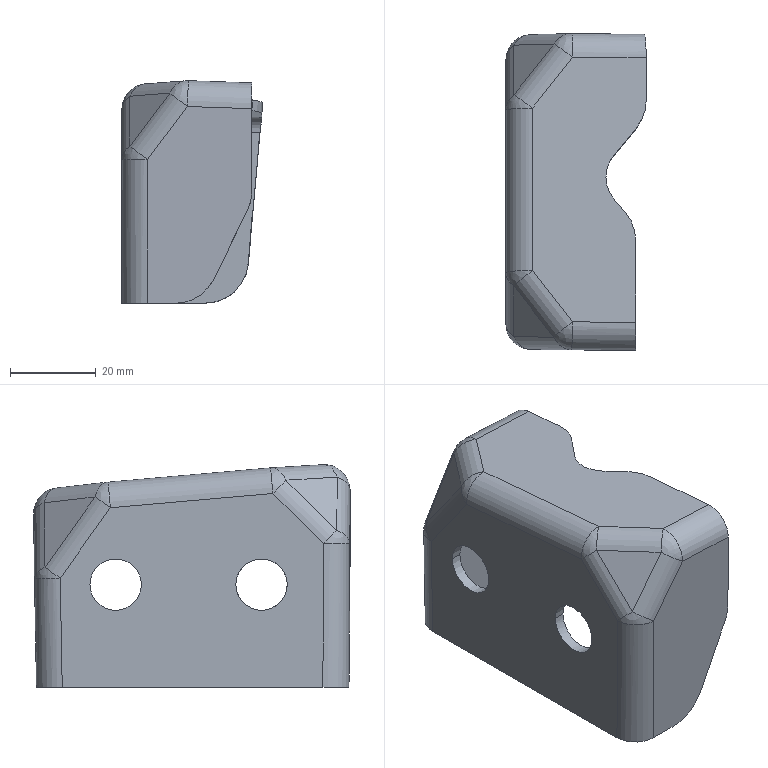Part | 1 solid | 70 faces | box 32.715 x 73.833 x 51.889 mm | volume 17818 mm3 | cylinder 26 | spline 26 | sphere 12 | plane 6 | commonest cylinder face diameters 12 x15 7 x11